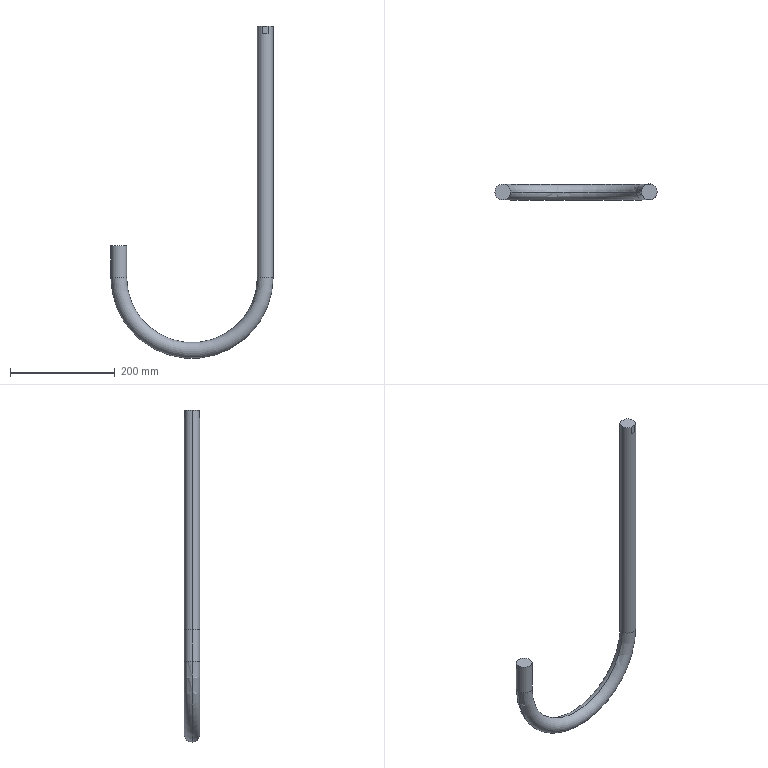Part | SolidWorks | features BaseBody 1 | 1 solid | 12 faces | box 310 x 30 x 635 mm | volume 692379 mm3 | plane 6 | cylinder 4 | torus 2 | commonest cylinder face diameters 30 x4
STEP:
#1=CARTESIAN_POINT('',(15.,0.,-480.));
#2=VERTEX_POINT('',#1);
#3=CARTESIAN_POINT('',(-15.,0.,-480.));
#4=VERTEX_POINT('',#3);
#5=CARTESIAN_POINT('',(0.,0.,-480.));
#6=DIRECTION('',(0.,0.,1.));
#7=DIRECTION('',(1.,0.,0.));
#8=AXIS2_PLACEMENT_3D('',#5,#6,#7);
#9=CIRCLE('',#8,15.);
#10=EDGE_CURVE('',#2,#4,#9,.T.);
#11=ORIENTED_EDGE('',*,*,#10,.F.);
#12=CARTESIAN_POINT('',(-295.,0.,-480.));
#13=VERTEX_POINT('',#12);
#14=CARTESIAN_POINT('',(-140.,0.,-480.));
#15=DIRECTION('',(0.,1.,0.));
#16=DIRECTION('',(0.,0.,1.));
#17=AXIS2_PLACEMENT_3D('',#14,#15,#16);
#18=CIRCLE('',#17,155.);
#19=EDGE_CURVE('',#2,#13,#18,.T.);
#20=ORIENTED_EDGE('',*,*,#19,.T.);
#21=CARTESIAN_POINT('',(-265.,0.,-480.));
#22=VERTEX_POINT('',#21);
#23=CARTESIAN_POINT('',(-280.,0.,-480.));
#24=DIRECTION('',(0.,0.,-1.));
#25=DIRECTION('',(-1.,0.,0.));
#26=AXIS2_PLACEMENT_3D('',#23,#24,#25);
#27=CIRCLE('',#26,15.);
#28=EDGE_CURVE('',#13,#22,#27,.T.);
#29=ORIENTED_EDGE('',*,*,#28,.T.);
#30=CARTESIAN_POINT('',(-140.,0.,-480.));
#31=DIRECTION('',(0.,1.,0.));
#32=DIRECTION('',(0.,0.,1.));
#33=AXIS2_PLACEMENT_3D('',#30,#31,#32);
#34=CIRCLE('',#33,125.);
#35=EDGE_CURVE('',#4,#22,#34,.T.);
#36=ORIENTED_EDGE('',*,*,#35,.F.);
#37=EDGE_LOOP('',(#11,#20,#29,#36));
#38=FACE_OUTER_BOUND('',#37,.T.);
#39=CARTESIAN_POINT('',(-140.,0.,-480.));
#40=DIRECTION('',(0.,1.,0.));
#41=DIRECTION('',(0.,0.,1.));
#42=AXIS2_PLACEMENT_3D('',#39,#40,#41);
#43=TOROIDAL_SURFACE('',#42,140.,15.);
#44=ADVANCED_FACE('',(#38),#43,.T.);
#45=ORIENTED_EDGE('',*,*,#28,.F.);
#46=CARTESIAN_POINT('',(-295.,0.,-420.));
#47=VERTEX_POINT('',#46);
#48=CARTESIAN_POINT('',(-295.,0.,-480.));
#49=DIRECTION('',(0.,0.,1.));
#50=VECTOR('',#49,1000.);
#51=LINE('',#48,#50);
#52=EDGE_CURVE('',#13,#47,#51,.T.);
#53=ORIENTED_EDGE('',*,*,#52,.T.);
#54=CARTESIAN_POINT('',(-265.,0.,-420.));
#55=VERTEX_POINT('',#54);
#56=CARTESIAN_POINT('',(-280.,0.,-420.));
#57=DIRECTION('',(0.,0.,-1.));
#58=DIRECTION('',(-1.,0.,0.));
#59=AXIS2_PLACEMENT_3D('',#56,#57,#58);
#60=CIRCLE('',#59,15.);
#61=EDGE_CURVE('',#47,#55,#60,.T.);
#62=ORIENTED_EDGE('',*,*,#61,.T.);
#63=CARTESIAN_POINT('',(-265.,0.,-480.));
#64=DIRECTION('',(0.,0.,1.));
#65=VECTOR('',#64,1000.);
#66=LINE('',#63,#65);
#67=EDGE_CURVE('',#22,#55,#66,.T.);
#68=ORIENTED_EDGE('',*,*,#67,.F.);
#69=EDGE_LOOP('',(#45,#53,#62,#68));
#70=FACE_OUTER_BOUND('',#69,.T.);
#71=CARTESIAN_POINT('',(-280.,0.,-480.));
#72=DIRECTION('',(0.,0.,1.));
#73=DIRECTION('',(1.,0.,0.));
#74=AXIS2_PLACEMENT_3D('',#71,#72,#73);
#75=CYLINDRICAL_SURFACE('',#74,15.);
#76=ADVANCED_FACE('',(#70),#75,.T.);
#77=CARTESIAN_POINT('',(15.,0.,0.));
#78=VERTEX_POINT('',#77);
#79=CARTESIAN_POINT('',(5.385,14.,0.));
#80=VERTEX_POINT('',#79);
#81=CARTESIAN_POINT('',(0.,0.,0.));
#82=DIRECTION('',(0.,0.,1.));
#83=DIRECTION('',(1.,0.,0.));
#84=AXIS2_PLACEMENT_3D('',#81,#82,#83);
#85=CIRCLE('',#84,15.);
#86=EDGE_CURVE('',#78,#80,#85,.T.);
#87=ORIENTED_EDGE('',*,*,#86,.F.);
#88=CARTESIAN_POINT('',(15.,0.,0.));
#89=DIRECTION('',(0.,0.,-1.));
#90=VECTOR('',#89,1000.);
#91=LINE('',#88,#90);
#92=EDGE_CURVE('',#78,#2,#91,.T.);
#93=ORIENTED_EDGE('',*,*,#92,.T.);
#94=ORIENTED_EDGE('',*,*,#10,.T.);
#95=CARTESIAN_POINT('',(-15.,0.,0.));
#96=VERTEX_POINT('',#95);
#97=CARTESIAN_POINT('',(-15.,0.,0.));
#98=DIRECTION('',(0.,0.,-1.));
#99=VECTOR('',#98,1000.);
#100=LINE('',#97,#99);
#101=EDGE_CURVE('',#96,#4,#100,.T.);
#102=ORIENTED_EDGE('',*,*,#101,.F.);
#103=CARTESIAN_POINT('',(-5.385,14.,0.));
#104=VERTEX_POINT('',#103);
#105=CARTESIAN_POINT('',(0.,0.,0.));
#106=DIRECTION('',(0.,0.,1.));
#107=DIRECTION('',(1.,0.,0.));
#108=AXIS2_PLACEMENT_3D('',#105,#106,#107);
#109=CIRCLE('',#108,15.);
#110=EDGE_CURVE('',#104,#96,#109,.T.);
#111=ORIENTED_EDGE('',*,*,#110,.F.);
#112=CARTESIAN_POINT('',(-5.385,14.,-15.));
#113=VERTEX_POINT('',#112);
#114=CARTESIAN_POINT('',(-5.385,14.,0.));
#115=DIRECTION('',(0.,0.,-1.));
#116=VECTOR('',#115,1000.);
#117=LINE('',#114,#116);
#118=EDGE_CURVE('',#104,#113,#117,.T.);
#119=ORIENTED_EDGE('',*,*,#118,.T.);
#120=CARTESIAN_POINT('',(5.385,14.,-15.));
#121=VERTEX_POINT('',#120);
#122=CARTESIAN_POINT('',(0.,0.,-15.));
#123=DIRECTION('',(0.,0.,-1.));
#124=DIRECTION('',(-1.,0.,0.));
#125=AXIS2_PLACEMENT_3D('',#122,#123,#124);
#126=CIRCLE('',#125,15.);
#127=EDGE_CURVE('',#113,#121,#126,.T.);
#128=ORIENTED_EDGE('',*,*,#127,.T.);
#129=CARTESIAN_POINT('',(5.385,14.,0.));
#130=DIRECTION('',(0.,0.,1.));
#131=VECTOR('',#130,1000.);
#132=LINE('',#129,#131);
#133=EDGE_CURVE('',#121,#80,#132,.T.);
#134=ORIENTED_EDGE('',*,*,#133,.T.);
#135=EDGE_LOOP('',(#87,#93,#94,#102,#111,#119,#128,#134));
#136=FACE_OUTER_BOUND('',#135,.T.);
#137=CARTESIAN_POINT('',(0.,0.,0.));
#138=DIRECTION('',(0.,0.,-1.));
#139=DIRECTION('',(-1.,0.,0.));
#140=AXIS2_PLACEMENT_3D('',#137,#138,#139);
#141=CYLINDRICAL_SURFACE('',#140,15.);
#142=ADVANCED_FACE('',(#136),#141,.T.);
#143=CARTESIAN_POINT('',(-5.385,-14.,0.));
#144=VERTEX_POINT('',#143);
#145=CARTESIAN_POINT('',(5.385,-14.,0.));
#146=VERTEX_POINT('',#145);
#147=CARTESIAN_POINT('',(-15.,-14.,0.));
#148=DIRECTION('',(1.,0.,0.));
#149=VECTOR('',#148,1000.);
#150=LINE('',#147,#149);
#151=EDGE_CURVE('',#144,#146,#150,.T.);
#152=ORIENTED_EDGE('',*,*,#151,.F.);
#153=CARTESIAN_POINT('',(-5.385,-14.,-15.));
#154=VERTEX_POINT('',#153);
#155=CARTESIAN_POINT('',(-5.385,-14.,0.));
#156=DIRECTION('',(0.,0.,1.));
#157=VECTOR('',#156,1000.);
#158=LINE('',#155,#157);
#159=EDGE_CURVE('',#154,#144,#158,.T.);
#160=ORIENTED_EDGE('',*,*,#159,.F.);
#161=CARTESIAN_POINT('',(5.385,-14.,-15.));
#162=VERTEX_POINT('',#161);
#163=CARTESIAN_POINT('',(-15.,-14.,-15.));
#164=DIRECTION('',(-1.,0.,0.));
#165=VECTOR('',#164,1000.);
#166=LINE('',#163,#165);
#167=EDGE_CURVE('',#162,#154,#166,.T.);
#168=ORIENTED_EDGE('',*,*,#167,.F.);
#169=CARTESIAN_POINT('',(5.385,-14.,0.));
#170=DIRECTION('',(0.,0.,-1.));
#171=VECTOR('',#170,1000.);
#172=LINE('',#169,#171);
#173=EDGE_CURVE('',#146,#162,#172,.T.);
#174=ORIENTED_EDGE('',*,*,#173,.F.);
#175=EDGE_LOOP('',(#152,#160,#168,#174));
#176=FACE_OUTER_BOUND('',#175,.T.);
#177=CARTESIAN_POINT('',(0.,-14.,0.));
#178=DIRECTION('',(0.,1.,0.));
#179=DIRECTION('',(1.,0.,0.));
#180=AXIS2_PLACEMENT_3D('',#177,#178,#179);
#181=PLANE('',#180);
#182=ADVANCED_FACE('',(#176),#181,.F.);
#183=CARTESIAN_POINT('',(0.,0.,-15.));
#184=DIRECTION('',(0.,0.,1.));
#185=DIRECTION('',(1.,0.,0.));
#186=AXIS2_PLACEMENT_3D('',#183,#184,#185);
#187=CIRCLE('',#186,15.);
#188=EDGE_CURVE('',#154,#162,#187,.T.);
#189=ORIENTED_EDGE('',*,*,#188,.T.);
#190=ORIENTED_EDGE('',*,*,#167,.T.);
#191=EDGE_LOOP('',(#189,#190));
#192=FACE_OUTER_BOUND('',#191,.T.);
#193=CARTESIAN_POINT('',(-15.,-14.,-15.));
#194=DIRECTION('',(0.,0.,1.));
#195=DIRECTION('',(1.,0.,0.));
#196=AXIS2_PLACEMENT_3D('',#193,#194,#195);
#197=PLANE('',#196);
#198=ADVANCED_FACE('',(#192),#197,.T.);
#199=CARTESIAN_POINT('',(-15.,14.,0.));
#200=DIRECTION('',(1.,0.,0.));
#201=VECTOR('',#200,1000.);
#202=LINE('',#199,#201);
#203=EDGE_CURVE('',#104,#80,#202,.T.);
#204=ORIENTED_EDGE('',*,*,#203,.T.);
#205=ORIENTED_EDGE('',*,*,#133,.F.);
#206=CARTESIAN_POINT('',(-15.,14.,-15.));
#207=DIRECTION('',(-1.,0.,0.));
#208=VECTOR('',#207,1000.);
#209=LINE('',#206,#208);
#210=EDGE_CURVE('',#121,#113,#209,.T.);
#211=ORIENTED_EDGE('',*,*,#210,.T.);
#212=ORIENTED_EDGE('',*,*,#118,.F.);
#213=EDGE_LOOP('',(#204,#205,#211,#212));
#214=FACE_OUTER_BOUND('',#213,.T.);
#215=CARTESIAN_POINT('',(0.,14.,0.));
#216=DIRECTION('',(0.,-1.,0.));
#217=DIRECTION('',(0.,0.,-1.));
#218=AXIS2_PLACEMENT_3D('',#215,#216,#217);
#219=PLANE('',#218);
#220=ADVANCED_FACE('',(#214),#219,.F.);
#221=ORIENTED_EDGE('',*,*,#210,.F.);
#222=ORIENTED_EDGE('',*,*,#127,.F.);
#223=EDGE_LOOP('',(#221,#222));
#224=FACE_OUTER_BOUND('',#223,.T.);
#225=CARTESIAN_POINT('',(-15.,14.,-15.));
#226=DIRECTION('',(0.,0.,-1.));
#227=DIRECTION('',(0.,-1.,0.));
#228=AXIS2_PLACEMENT_3D('',#225,#226,#227);
#229=PLANE('',#228);
#230=ADVANCED_FACE('',(#224),#229,.F.);
#231=ORIENTED_EDGE('',*,*,#151,.T.);
#232=CARTESIAN_POINT('',(0.,0.,0.));
#233=DIRECTION('',(0.,0.,1.));
#234=DIRECTION('',(1.,0.,0.));
#235=AXIS2_PLACEMENT_3D('',#232,#233,#234);
#236=CIRCLE('',#235,15.);
#237=EDGE_CURVE('',#146,#78,#236,.T.);
#238=ORIENTED_EDGE('',*,*,#237,.T.);
#239=ORIENTED_EDGE('',*,*,#86,.T.);
#240=ORIENTED_EDGE('',*,*,#203,.F.);
#241=ORIENTED_EDGE('',*,*,#110,.T.);
#242=CARTESIAN_POINT('',(0.,0.,0.));
#243=DIRECTION('',(0.,0.,1.));
#244=DIRECTION('',(1.,0.,0.));
#245=AXIS2_PLACEMENT_3D('',#242,#243,#244);
#246=CIRCLE('',#245,15.);
#247=EDGE_CURVE('',#96,#144,#246,.T.);
#248=ORIENTED_EDGE('',*,*,#247,.T.);
#249=EDGE_LOOP('',(#231,#238,#239,#240,#241,#248));
#250=FACE_OUTER_BOUND('',#249,.T.);
#251=CARTESIAN_POINT('',(0.,0.,0.));
#252=DIRECTION('',(0.,0.,1.));
#253=DIRECTION('',(1.,0.,0.));
#254=AXIS2_PLACEMENT_3D('',#251,#252,#253);
#255=PLANE('',#254);
#256=ADVANCED_FACE('',(#250),#255,.T.);
#257=CARTESIAN_POINT('',(-280.,0.,-420.));
#258=DIRECTION('',(0.,0.,-1.));
#259=DIRECTION('',(-1.,0.,0.));
#260=AXIS2_PLACEMENT_3D('',#257,#258,#259);
#261=CIRCLE('',#260,15.);
#262=EDGE_CURVE('',#55,#47,#261,.T.);
#263=ORIENTED_EDGE('',*,*,#262,.F.);
#264=ORIENTED_EDGE('',*,*,#61,.F.);
#265=EDGE_LOOP('',(#263,#264));
#266=FACE_OUTER_BOUND('',#265,.T.);
#267=CARTESIAN_POINT('',(-280.,0.,-420.));
#268=DIRECTION('',(0.,0.,-1.));
#269=DIRECTION('',(0.,-1.,0.));
#270=AXIS2_PLACEMENT_3D('',#267,#268,#269);
#271=PLANE('',#270);
#272=ADVANCED_FACE('',(#266),#271,.F.);
#273=ORIENTED_EDGE('',*,*,#92,.F.);
#274=ORIENTED_EDGE('',*,*,#237,.F.);
#275=ORIENTED_EDGE('',*,*,#173,.T.);
#276=ORIENTED_EDGE('',*,*,#188,.F.);
#277=ORIENTED_EDGE('',*,*,#159,.T.);
#278=ORIENTED_EDGE('',*,*,#247,.F.);
#279=ORIENTED_EDGE('',*,*,#101,.T.);
#280=CARTESIAN_POINT('',(0.,0.,-480.));
#281=DIRECTION('',(0.,0.,1.));
#282=DIRECTION('',(1.,0.,0.));
#283=AXIS2_PLACEMENT_3D('',#280,#281,#282);
#284=CIRCLE('',#283,15.);
#285=EDGE_CURVE('',#4,#2,#284,.T.);
#286=ORIENTED_EDGE('',*,*,#285,.T.);
#287=EDGE_LOOP('',(#273,#274,#275,#276,#277,#278,#279,#286));
#288=FACE_OUTER_BOUND('',#287,.T.);
#289=CARTESIAN_POINT('',(0.,0.,0.));
#290=DIRECTION('',(0.,0.,-1.));
#291=DIRECTION('',(-1.,0.,0.));
#292=AXIS2_PLACEMENT_3D('',#289,#290,#291);
#293=CYLINDRICAL_SURFACE('',#292,15.);
#294=ADVANCED_FACE('',(#288),#293,.T.);
#295=ORIENTED_EDGE('',*,*,#52,.F.);
#296=CARTESIAN_POINT('',(-280.,0.,-480.));
#297=DIRECTION('',(0.,0.,-1.));
#298=DIRECTION('',(-1.,0.,0.));
#299=AXIS2_PLACEMENT_3D('',#296,#297,#298);
#300=CIRCLE('',#299,15.);
#301=EDGE_CURVE('',#22,#13,#300,.T.);
#302=ORIENTED_EDGE('',*,*,#301,.F.);
#303=ORIENTED_EDGE('',*,*,#67,.T.);
#304=ORIENTED_EDGE('',*,*,#262,.T.);
#305=EDGE_LOOP('',(#295,#302,#303,#304));
#306=FACE_OUTER_BOUND('',#305,.T.);
#307=CARTESIAN_POINT('',(-280.,0.,-480.));
#308=DIRECTION('',(0.,0.,1.));
#309=DIRECTION('',(1.,0.,0.));
#310=AXIS2_PLACEMENT_3D('',#307,#308,#309);
#311=CYLINDRICAL_SURFACE('',#310,15.);
#312=ADVANCED_FACE('',(#306),#311,.T.);
#313=ORIENTED_EDGE('',*,*,#19,.F.);
#314=ORIENTED_EDGE('',*,*,#285,.F.);
#315=ORIENTED_EDGE('',*,*,#35,.T.);
#316=ORIENTED_EDGE('',*,*,#301,.T.);
#317=EDGE_LOOP('',(#313,#314,#315,#316));
#318=FACE_OUTER_BOUND('',#317,.T.);
#319=CARTESIAN_POINT('',(-140.,0.,-480.));
#320=DIRECTION('',(0.,1.,0.));
#321=DIRECTION('',(0.,0.,1.));
#322=AXIS2_PLACEMENT_3D('',#319,#320,#321);
#323=TOROIDAL_SURFACE('',#322,140.,15.);
#324=ADVANCED_FACE('',(#318),#323,.T.);
#325=CLOSED_SHELL('',(#44,#76,#142,#182,#198,#220,#230,#256,#272,#294,#312,#324));
#326=MANIFOLD_SOLID_BREP('',#325);
#327=CARTESIAN_POINT('',(0.,0.,0.));
#328=DIRECTION('',(0.,0.,1.));
#329=DIRECTION('',(1.,0.,0.));
#330=AXIS2_PLACEMENT_3D('',#327,#328,#329);
#331=(LENGTH_UNIT()NAMED_UNIT(*)SI_UNIT(.MILLI.,.METRE.));
#332=UNCERTAINTY_MEASURE_WITH_UNIT(LENGTH_MEASURE(0.00001),#331,'','');
#333=(NAMED_UNIT(*)PLANE_ANGLE_UNIT()SI_UNIT($,.RADIAN.));
#334=(NAMED_UNIT(*)SI_UNIT($,.STERADIAN.)SOLID_ANGLE_UNIT());
#335=(GEOMETRIC_REPRESENTATION_CONTEXT(3)GLOBAL_UNCERTAINTY_ASSIGNED_CONTEXT((#332))GLOBAL_UNIT_ASSIGNED_CONTEXT((#331,#333,#334))REPRESENTATION_CONTEXT('',''));
#336=ADVANCED_BREP_SHAPE_REPRESENTATION('',(#326,#330),#335);